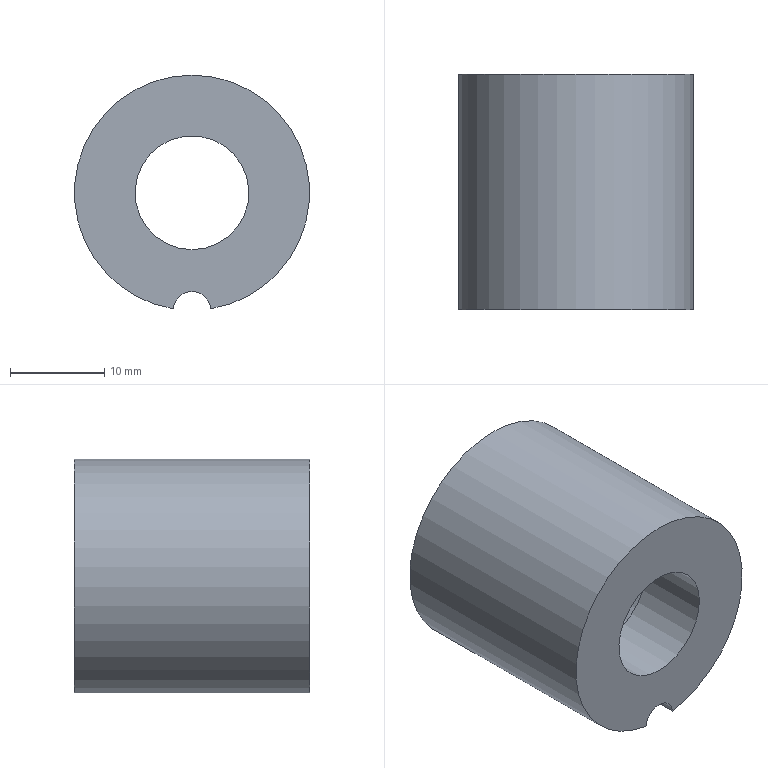Part | NX | features solid 2 | 1 solid | 7 faces | box 25 x 25 x 24.84 mm | volume 7521 mm3 | cylinder 4 | plane 3 | commonest cylinder face diameters 4 x1 12.1 x1 16.6 x1 25 x1
STEP:
#1=CARTESIAN_POINT('',(-496.002,-474.808,-12.1));
#2=VERTEX_POINT('',#1);
#3=CARTESIAN_POINT('',(-496.002,-499.808,-12.1));
#4=VERTEX_POINT('',#3);
#5=CARTESIAN_POINT('',(-496.002,-487.308,-12.1));
#6=DIRECTION('',(0.,-1.,0.));
#7=VECTOR('',#6,1000.);
#8=LINE('',#5,#7);
#9=EDGE_CURVE('',#2,#4,#8,.T.);
#10=ORIENTED_EDGE('',*,*,#9,.T.);
#11=CARTESIAN_POINT('',(-492.015,-499.808,-12.1));
#12=VERTEX_POINT('',#11);
#13=CARTESIAN_POINT('',(-494.009,-499.808,0.2395));
#14=DIRECTION('',(0.,1.,0.));
#15=DIRECTION('',(0.,0.,-1.));
#16=AXIS2_PLACEMENT_3D('',#13,#14,#15);
#17=CIRCLE('',#16,12.5);
#18=EDGE_CURVE('',#4,#12,#17,.T.);
#19=ORIENTED_EDGE('',*,*,#18,.T.);
#20=CARTESIAN_POINT('',(-492.015,-474.808,-12.1));
#21=VERTEX_POINT('',#20);
#22=CARTESIAN_POINT('',(-492.015,-487.308,-12.1));
#23=DIRECTION('',(0.,-1.,0.));
#24=VECTOR('',#23,1000.);
#25=LINE('',#22,#24);
#26=EDGE_CURVE('',#12,#21,#25,.F.);
#27=ORIENTED_EDGE('',*,*,#26,.T.);
#28=CARTESIAN_POINT('',(-494.009,-474.808,0.2395));
#29=DIRECTION('',(0.,1.,0.));
#30=DIRECTION('',(0.,0.,-1.));
#31=AXIS2_PLACEMENT_3D('',#28,#29,#30);
#32=CIRCLE('',#31,12.5);
#33=EDGE_CURVE('',#2,#21,#32,.T.);
#34=ORIENTED_EDGE('',*,*,#33,.F.);
#35=EDGE_LOOP('',(#10,#19,#27,#34));
#36=FACE_BOUND('',#35,.T.);
#37=CARTESIAN_POINT('',(-494.009,-474.808,0.2395));
#38=DIRECTION('',(0.,-1.,0.));
#39=DIRECTION('',(0.,0.,-1.));
#40=AXIS2_PLACEMENT_3D('',#37,#38,#39);
#41=CYLINDRICAL_SURFACE('',#40,12.5);
#42=ADVANCED_FACE('',(#36),#41,.T.);
#43=CARTESIAN_POINT('',(-494.009,-474.808,-8.06));
#44=VERTEX_POINT('',#43);
#45=CARTESIAN_POINT('',(-494.009,-474.808,0.2395));
#46=DIRECTION('',(0.,1.,0.));
#47=DIRECTION('',(0.,0.,-1.));
#48=AXIS2_PLACEMENT_3D('',#45,#46,#47);
#49=CIRCLE('',#48,8.3);
#50=EDGE_CURVE('',#44,#44,#49,.T.);
#51=ORIENTED_EDGE('',*,*,#50,.F.);
#52=EDGE_LOOP('',(#51));
#53=FACE_BOUND('',#52,.T.);
#54=ORIENTED_EDGE('',*,*,#33,.T.);
#55=CARTESIAN_POINT('',(-494.009,-474.808,-12.26));
#56=DIRECTION('',(0.,1.,0.));
#57=DIRECTION('',(0.,0.,-1.));
#58=AXIS2_PLACEMENT_3D('',#55,#56,#57);
#59=CIRCLE('',#58,2.);
#60=EDGE_CURVE('',#2,#21,#59,.T.);
#61=ORIENTED_EDGE('',*,*,#60,.F.);
#62=EDGE_LOOP('',(#54,#61));
#63=FACE_BOUND('',#62,.T.);
#64=CARTESIAN_POINT('',(-494.009,-474.808,0.2395));
#65=DIRECTION('',(0.,-1.,0.));
#66=DIRECTION('',(0.,0.,-1.));
#67=AXIS2_PLACEMENT_3D('',#64,#65,#66);
#68=PLANE('',#67);
#69=ADVANCED_FACE('',(#53,#63),#68,.F.);
#70=CARTESIAN_POINT('',(-494.009,-499.808,-5.81));
#71=VERTEX_POINT('',#70);
#72=CARTESIAN_POINT('',(-494.009,-499.808,0.2395));
#73=DIRECTION('',(0.,1.,0.));
#74=DIRECTION('',(0.,0.,-1.));
#75=AXIS2_PLACEMENT_3D('',#72,#73,#74);
#76=CIRCLE('',#75,6.05);
#77=EDGE_CURVE('',#71,#71,#76,.T.);
#78=ORIENTED_EDGE('',*,*,#77,.T.);
#79=EDGE_LOOP('',(#78));
#80=FACE_BOUND('',#79,.T.);
#81=CARTESIAN_POINT('',(-494.009,-499.808,-12.26));
#82=DIRECTION('',(0.,1.,0.));
#83=DIRECTION('',(0.,0.,-1.));
#84=AXIS2_PLACEMENT_3D('',#81,#82,#83);
#85=CIRCLE('',#84,2.);
#86=EDGE_CURVE('',#4,#12,#85,.T.);
#87=ORIENTED_EDGE('',*,*,#86,.T.);
#88=ORIENTED_EDGE('',*,*,#18,.F.);
#89=EDGE_LOOP('',(#87,#88));
#90=FACE_BOUND('',#89,.T.);
#91=CARTESIAN_POINT('',(-494.009,-499.808,0.2395));
#92=DIRECTION('',(0.,-1.,0.));
#93=DIRECTION('',(0.,0.,-1.));
#94=AXIS2_PLACEMENT_3D('',#91,#92,#93);
#95=PLANE('',#94);
#96=ADVANCED_FACE('',(#80,#90),#95,.T.);
#97=ORIENTED_EDGE('',*,*,#50,.T.);
#98=EDGE_LOOP('',(#97));
#99=FACE_BOUND('',#98,.T.);
#100=CARTESIAN_POINT('',(-494.009,-491.808,-8.06));
#101=VERTEX_POINT('',#100);
#102=CARTESIAN_POINT('',(-494.009,-491.808,0.2395));
#103=DIRECTION('',(0.,1.,0.));
#104=DIRECTION('',(0.,0.,-1.));
#105=AXIS2_PLACEMENT_3D('',#102,#103,#104);
#106=CIRCLE('',#105,8.3);
#107=EDGE_CURVE('',#101,#101,#106,.T.);
#108=ORIENTED_EDGE('',*,*,#107,.F.);
#109=EDGE_LOOP('',(#108));
#110=FACE_BOUND('',#109,.T.);
#111=CARTESIAN_POINT('',(-494.009,-474.808,0.2395));
#112=DIRECTION('',(0.,-1.,0.));
#113=DIRECTION('',(0.,0.,-1.));
#114=AXIS2_PLACEMENT_3D('',#111,#112,#113);
#115=CYLINDRICAL_SURFACE('',#114,8.3);
#116=ADVANCED_FACE('',(#99,#110),#115,.F.);
#117=CARTESIAN_POINT('',(-494.009,-491.808,-5.81));
#118=VERTEX_POINT('',#117);
#119=CARTESIAN_POINT('',(-494.009,-491.808,0.2395));
#120=DIRECTION('',(0.,1.,0.));
#121=DIRECTION('',(0.,0.,-1.));
#122=AXIS2_PLACEMENT_3D('',#119,#120,#121);
#123=CIRCLE('',#122,6.05);
#124=EDGE_CURVE('',#118,#118,#123,.T.);
#125=ORIENTED_EDGE('',*,*,#124,.F.);
#126=EDGE_LOOP('',(#125));
#127=FACE_BOUND('',#126,.T.);
#128=ORIENTED_EDGE('',*,*,#107,.T.);
#129=EDGE_LOOP('',(#128));
#130=FACE_BOUND('',#129,.T.);
#131=CARTESIAN_POINT('',(-494.009,-491.808,0.2395));
#132=DIRECTION('',(0.,-1.,0.));
#133=DIRECTION('',(0.,0.,-1.));
#134=AXIS2_PLACEMENT_3D('',#131,#132,#133);
#135=PLANE('',#134);
#136=ADVANCED_FACE('',(#127,#130),#135,.F.);
#137=ORIENTED_EDGE('',*,*,#9,.F.);
#138=ORIENTED_EDGE('',*,*,#60,.T.);
#139=ORIENTED_EDGE('',*,*,#26,.F.);
#140=ORIENTED_EDGE('',*,*,#86,.F.);
#141=EDGE_LOOP('',(#137,#138,#139,#140));
#142=FACE_BOUND('',#141,.T.);
#143=CARTESIAN_POINT('',(-494.009,-474.808,-12.26));
#144=DIRECTION('',(0.,-1.,0.));
#145=DIRECTION('',(0.,0.,-1.));
#146=AXIS2_PLACEMENT_3D('',#143,#144,#145);
#147=CYLINDRICAL_SURFACE('',#146,2.);
#148=ADVANCED_FACE('',(#142),#147,.F.);
#149=ORIENTED_EDGE('',*,*,#77,.F.);
#150=EDGE_LOOP('',(#149));
#151=FACE_BOUND('',#150,.T.);
#152=ORIENTED_EDGE('',*,*,#124,.T.);
#153=EDGE_LOOP('',(#152));
#154=FACE_BOUND('',#153,.T.);
#155=CARTESIAN_POINT('',(-494.009,-474.808,0.2395));
#156=DIRECTION('',(0.,-1.,0.));
#157=DIRECTION('',(0.,0.,-1.));
#158=AXIS2_PLACEMENT_3D('',#155,#156,#157);
#159=CYLINDRICAL_SURFACE('',#158,6.05);
#160=ADVANCED_FACE('',(#151,#154),#159,.F.);
#161=CLOSED_SHELL('',(#42,#69,#96,#116,#136,#148,#160));
#162=MANIFOLD_SOLID_BREP('',#161);
#163=(LENGTH_UNIT()NAMED_UNIT(*)SI_UNIT(.MILLI.,.METRE.));
#164=UNCERTAINTY_MEASURE_WITH_UNIT(LENGTH_MEASURE(0.00001),#163,'','');
#165=(NAMED_UNIT(*)PLANE_ANGLE_UNIT()SI_UNIT($,.RADIAN.));
#166=(NAMED_UNIT(*)SI_UNIT($,.STERADIAN.)SOLID_ANGLE_UNIT());
#167=(GEOMETRIC_REPRESENTATION_CONTEXT(3)GLOBAL_UNCERTAINTY_ASSIGNED_CONTEXT((#164))GLOBAL_UNIT_ASSIGNED_CONTEXT((#163,#165,#166))REPRESENTATION_CONTEXT('',''));
#168=ADVANCED_BREP_SHAPE_REPRESENTATION('',(#162),#167);